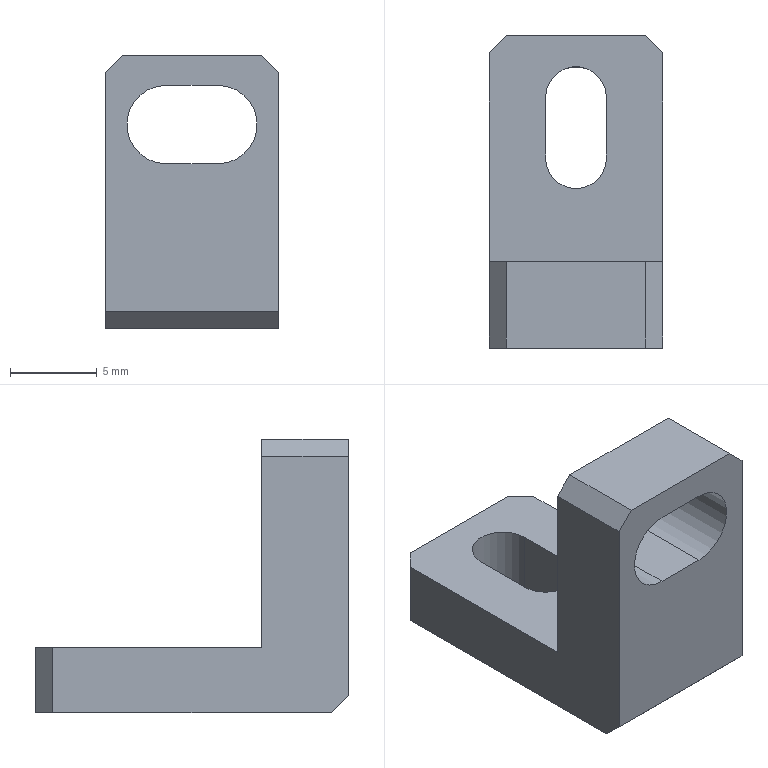Part | SolidWorks | features ICE 4, Chamfer 1, Extrusion 1 | 1 solid | 21 faces | box 10 x 18 x 15.75 mm | volume 1032 mm3 | plane 17 | cylinder 4 | commonest cylinder face diameters 3.5 x2 4.5 x2
STEP:
#1=CARTESIAN_POINT('',(0.,17.,-3.75));
#2=VERTEX_POINT('',#1);
#3=CARTESIAN_POINT('',(0.,1.,-3.75));
#4=VERTEX_POINT('',#3);
#5=CARTESIAN_POINT('',(0.,18.,-3.75));
#6=DIRECTION('',(0.,-1.,0.));
#7=VECTOR('',#6,1000.);
#8=LINE('',#5,#7);
#9=EDGE_CURVE('',#2,#4,#8,.T.);
#10=ORIENTED_EDGE('',*,*,#9,.T.);
#11=CARTESIAN_POINT('',(0.,0.,-2.75));
#12=VERTEX_POINT('',#11);
#13=CARTESIAN_POINT('',(0.,1.,-3.75));
#14=DIRECTION('',(0.,-0.7071,0.7071));
#15=VECTOR('',#14,1000.);
#16=LINE('',#13,#15);
#17=EDGE_CURVE('',#4,#12,#16,.T.);
#18=ORIENTED_EDGE('',*,*,#17,.T.);
#19=CARTESIAN_POINT('',(0.,0.,11.));
#20=VERTEX_POINT('',#19);
#21=CARTESIAN_POINT('',(0.,0.,0.));
#22=DIRECTION('',(0.,0.,1.));
#23=VECTOR('',#22,1000.);
#24=LINE('',#21,#23);
#25=EDGE_CURVE('',#12,#20,#24,.T.);
#26=ORIENTED_EDGE('',*,*,#25,.T.);
#27=CARTESIAN_POINT('',(0.,5.,11.));
#28=VERTEX_POINT('',#27);
#29=CARTESIAN_POINT('',(0.,5.,11.));
#30=DIRECTION('',(0.,1.,0.));
#31=VECTOR('',#30,1000.);
#32=LINE('',#29,#31);
#33=EDGE_CURVE('',#20,#28,#32,.T.);
#34=ORIENTED_EDGE('',*,*,#33,.T.);
#35=CARTESIAN_POINT('',(0.,5.,0.));
#36=VERTEX_POINT('',#35);
#37=CARTESIAN_POINT('',(0.,5.,0.));
#38=DIRECTION('',(0.,0.,-1.));
#39=VECTOR('',#38,1000.);
#40=LINE('',#37,#39);
#41=EDGE_CURVE('',#28,#36,#40,.T.);
#42=ORIENTED_EDGE('',*,*,#41,.T.);
#43=CARTESIAN_POINT('',(0.,17.,0.));
#44=VERTEX_POINT('',#43);
#45=CARTESIAN_POINT('',(0.,18.,0.));
#46=DIRECTION('',(0.,-1.,0.));
#47=VECTOR('',#46,1000.);
#48=LINE('',#45,#47);
#49=EDGE_CURVE('',#44,#36,#48,.T.);
#50=ORIENTED_EDGE('',*,*,#49,.F.);
#51=CARTESIAN_POINT('',(0.,17.,0.));
#52=DIRECTION('',(0.,0.,-1.));
#53=VECTOR('',#52,1000.);
#54=LINE('',#51,#53);
#55=EDGE_CURVE('',#44,#2,#54,.T.);
#56=ORIENTED_EDGE('',*,*,#55,.T.);
#57=EDGE_LOOP('',(#10,#18,#26,#34,#42,#50,#56));
#58=FACE_OUTER_BOUND('',#57,.T.);
#59=CARTESIAN_POINT('',(0.,18.,0.));
#60=DIRECTION('',(1.,0.,0.));
#61=DIRECTION('',(0.,0.,-1.));
#62=AXIS2_PLACEMENT_3D('',#59,#60,#61);
#63=PLANE('',#62);
#64=ADVANCED_FACE('',(#58),#63,.F.);
#65=CARTESIAN_POINT('',(3.25,14.45,0.));
#66=VERTEX_POINT('',#65);
#67=CARTESIAN_POINT('',(3.25,10.95,0.));
#68=VERTEX_POINT('',#67);
#69=CARTESIAN_POINT('',(3.25,14.45,0.));
#70=DIRECTION('',(0.,-1.,0.));
#71=VECTOR('',#70,1000.);
#72=LINE('',#69,#71);
#73=EDGE_CURVE('',#66,#68,#72,.T.);
#74=ORIENTED_EDGE('',*,*,#73,.F.);
#75=CARTESIAN_POINT('',(6.75,14.45,0.));
#76=VERTEX_POINT('',#75);
#77=CARTESIAN_POINT('',(5.,14.45,0.));
#78=DIRECTION('',(0.,0.,1.));
#79=DIRECTION('',(1.,0.,0.));
#80=AXIS2_PLACEMENT_3D('',#77,#78,#79);
#81=CIRCLE('',#80,1.75);
#82=EDGE_CURVE('',#76,#66,#81,.T.);
#83=ORIENTED_EDGE('',*,*,#82,.F.);
#84=CARTESIAN_POINT('',(6.75,10.95,0.));
#85=VERTEX_POINT('',#84);
#86=CARTESIAN_POINT('',(6.75,14.45,0.));
#87=DIRECTION('',(0.,1.,0.));
#88=VECTOR('',#87,1000.);
#89=LINE('',#86,#88);
#90=EDGE_CURVE('',#85,#76,#89,.T.);
#91=ORIENTED_EDGE('',*,*,#90,.F.);
#92=CARTESIAN_POINT('',(5.,10.95,0.));
#93=DIRECTION('',(0.,0.,1.));
#94=DIRECTION('',(1.,0.,0.));
#95=AXIS2_PLACEMENT_3D('',#92,#93,#94);
#96=CIRCLE('',#95,1.75);
#97=EDGE_CURVE('',#68,#85,#96,.T.);
#98=ORIENTED_EDGE('',*,*,#97,.F.);
#99=EDGE_LOOP('',(#74,#83,#91,#98));
#100=FACE_BOUND('',#99,.T.);
#101=CARTESIAN_POINT('',(10.,17.,0.));
#102=VERTEX_POINT('',#101);
#103=CARTESIAN_POINT('',(10.,5.,0.));
#104=VERTEX_POINT('',#103);
#105=CARTESIAN_POINT('',(10.,18.,0.));
#106=DIRECTION('',(0.,-1.,0.));
#107=VECTOR('',#106,1000.);
#108=LINE('',#105,#107);
#109=EDGE_CURVE('',#102,#104,#108,.T.);
#110=ORIENTED_EDGE('',*,*,#109,.F.);
#111=CARTESIAN_POINT('',(9.,18.,0.));
#112=VERTEX_POINT('',#111);
#113=CARTESIAN_POINT('',(9.,18.,0.));
#114=DIRECTION('',(-0.7071,0.7071,0.));
#115=VECTOR('',#114,1000.);
#116=LINE('',#113,#115);
#117=EDGE_CURVE('',#102,#112,#116,.T.);
#118=ORIENTED_EDGE('',*,*,#117,.T.);
#119=CARTESIAN_POINT('',(1.,18.,0.));
#120=VERTEX_POINT('',#119);
#121=CARTESIAN_POINT('',(0.,18.,0.));
#122=DIRECTION('',(1.,0.,0.));
#123=VECTOR('',#122,1000.);
#124=LINE('',#121,#123);
#125=EDGE_CURVE('',#120,#112,#124,.T.);
#126=ORIENTED_EDGE('',*,*,#125,.F.);
#127=CARTESIAN_POINT('',(1.,18.,0.));
#128=DIRECTION('',(-0.7071,-0.7071,0.));
#129=VECTOR('',#128,1000.);
#130=LINE('',#127,#129);
#131=EDGE_CURVE('',#120,#44,#130,.T.);
#132=ORIENTED_EDGE('',*,*,#131,.T.);
#133=ORIENTED_EDGE('',*,*,#49,.T.);
#134=CARTESIAN_POINT('',(0.,5.,0.));
#135=DIRECTION('',(1.,0.,0.));
#136=VECTOR('',#135,1000.);
#137=LINE('',#134,#136);
#138=EDGE_CURVE('',#36,#104,#137,.T.);
#139=ORIENTED_EDGE('',*,*,#138,.T.);
#140=EDGE_LOOP('',(#110,#118,#126,#132,#133,#139));
#141=FACE_OUTER_BOUND('',#140,.T.);
#142=CARTESIAN_POINT('',(0.,18.,0.));
#143=DIRECTION('',(0.,0.,-1.));
#144=DIRECTION('',(-1.,0.,0.));
#145=AXIS2_PLACEMENT_3D('',#142,#143,#144);
#146=PLANE('',#145);
#147=ADVANCED_FACE('',(#100,#141),#146,.F.);
#148=CARTESIAN_POINT('',(10.,0.,11.));
#149=VERTEX_POINT('',#148);
#150=CARTESIAN_POINT('',(10.,0.,-2.75));
#151=VERTEX_POINT('',#150);
#152=CARTESIAN_POINT('',(10.,0.,0.));
#153=DIRECTION('',(0.,0.,-1.));
#154=VECTOR('',#153,1000.);
#155=LINE('',#152,#154);
#156=EDGE_CURVE('',#149,#151,#155,.T.);
#157=ORIENTED_EDGE('',*,*,#156,.T.);
#158=CARTESIAN_POINT('',(10.,1.,-3.75));
#159=VERTEX_POINT('',#158);
#160=CARTESIAN_POINT('',(10.,1.,-3.75));
#161=DIRECTION('',(0.,0.7071,-0.7071));
#162=VECTOR('',#161,1000.);
#163=LINE('',#160,#162);
#164=EDGE_CURVE('',#151,#159,#163,.T.);
#165=ORIENTED_EDGE('',*,*,#164,.T.);
#166=CARTESIAN_POINT('',(10.,17.,-3.75));
#167=VERTEX_POINT('',#166);
#168=CARTESIAN_POINT('',(10.,18.,-3.75));
#169=DIRECTION('',(0.,-1.,0.));
#170=VECTOR('',#169,1000.);
#171=LINE('',#168,#170);
#172=EDGE_CURVE('',#167,#159,#171,.T.);
#173=ORIENTED_EDGE('',*,*,#172,.F.);
#174=CARTESIAN_POINT('',(10.,17.,0.));
#175=DIRECTION('',(0.,0.,1.));
#176=VECTOR('',#175,1000.);
#177=LINE('',#174,#176);
#178=EDGE_CURVE('',#167,#102,#177,.T.);
#179=ORIENTED_EDGE('',*,*,#178,.T.);
#180=ORIENTED_EDGE('',*,*,#109,.T.);
#181=CARTESIAN_POINT('',(10.,5.,11.));
#182=VERTEX_POINT('',#181);
#183=CARTESIAN_POINT('',(10.,5.,0.));
#184=DIRECTION('',(0.,0.,1.));
#185=VECTOR('',#184,1000.);
#186=LINE('',#183,#185);
#187=EDGE_CURVE('',#104,#182,#186,.T.);
#188=ORIENTED_EDGE('',*,*,#187,.T.);
#189=CARTESIAN_POINT('',(10.,0.,11.));
#190=DIRECTION('',(0.,-1.,0.));
#191=VECTOR('',#190,1000.);
#192=LINE('',#189,#191);
#193=EDGE_CURVE('',#182,#149,#192,.T.);
#194=ORIENTED_EDGE('',*,*,#193,.T.);
#195=EDGE_LOOP('',(#157,#165,#173,#179,#180,#188,#194));
#196=FACE_OUTER_BOUND('',#195,.T.);
#197=CARTESIAN_POINT('',(10.,18.,0.));
#198=DIRECTION('',(-1.,0.,0.));
#199=DIRECTION('',(0.,0.,1.));
#200=AXIS2_PLACEMENT_3D('',#197,#198,#199);
#201=PLANE('',#200);
#202=ADVANCED_FACE('',(#196),#201,.F.);
#203=CARTESIAN_POINT('',(6.75,10.95,-3.75));
#204=VERTEX_POINT('',#203);
#205=CARTESIAN_POINT('',(6.75,14.45,-3.75));
#206=VERTEX_POINT('',#205);
#207=CARTESIAN_POINT('',(6.75,18.,-3.75));
#208=DIRECTION('',(0.,1.,0.));
#209=VECTOR('',#208,1000.);
#210=LINE('',#207,#209);
#211=EDGE_CURVE('',#204,#206,#210,.T.);
#212=ORIENTED_EDGE('',*,*,#211,.T.);
#213=CARTESIAN_POINT('',(3.25,14.45,-3.75));
#214=VERTEX_POINT('',#213);
#215=CARTESIAN_POINT('',(5.,14.45,-3.75));
#216=DIRECTION('',(0.,0.,1.));
#217=DIRECTION('',(1.,0.,0.));
#218=AXIS2_PLACEMENT_3D('',#215,#216,#217);
#219=CIRCLE('',#218,1.75);
#220=EDGE_CURVE('',#206,#214,#219,.T.);
#221=ORIENTED_EDGE('',*,*,#220,.T.);
#222=CARTESIAN_POINT('',(3.25,10.95,-3.75));
#223=VERTEX_POINT('',#222);
#224=CARTESIAN_POINT('',(3.25,18.,-3.75));
#225=DIRECTION('',(0.,-1.,0.));
#226=VECTOR('',#225,1000.);
#227=LINE('',#224,#226);
#228=EDGE_CURVE('',#214,#223,#227,.T.);
#229=ORIENTED_EDGE('',*,*,#228,.T.);
#230=CARTESIAN_POINT('',(5.,10.95,-3.75));
#231=DIRECTION('',(0.,0.,1.));
#232=DIRECTION('',(1.,0.,0.));
#233=AXIS2_PLACEMENT_3D('',#230,#231,#232);
#234=CIRCLE('',#233,1.75);
#235=EDGE_CURVE('',#223,#204,#234,.T.);
#236=ORIENTED_EDGE('',*,*,#235,.T.);
#237=EDGE_LOOP('',(#212,#221,#229,#236));
#238=FACE_BOUND('',#237,.T.);
#239=ORIENTED_EDGE('',*,*,#172,.T.);
#240=CARTESIAN_POINT('',(0.,1.,-3.75));
#241=DIRECTION('',(-1.,0.,0.));
#242=VECTOR('',#241,1000.);
#243=LINE('',#240,#242);
#244=EDGE_CURVE('',#159,#4,#243,.T.);
#245=ORIENTED_EDGE('',*,*,#244,.T.);
#246=ORIENTED_EDGE('',*,*,#9,.F.);
#247=CARTESIAN_POINT('',(1.,18.,-3.75));
#248=VERTEX_POINT('',#247);
#249=CARTESIAN_POINT('',(1.,18.,-3.75));
#250=DIRECTION('',(0.7071,0.7071,0.));
#251=VECTOR('',#250,1000.);
#252=LINE('',#249,#251);
#253=EDGE_CURVE('',#2,#248,#252,.T.);
#254=ORIENTED_EDGE('',*,*,#253,.T.);
#255=CARTESIAN_POINT('',(9.,18.,-3.75));
#256=VERTEX_POINT('',#255);
#257=CARTESIAN_POINT('',(0.,18.,-3.75));
#258=DIRECTION('',(-1.,0.,0.));
#259=VECTOR('',#258,1000.);
#260=LINE('',#257,#259);
#261=EDGE_CURVE('',#256,#248,#260,.T.);
#262=ORIENTED_EDGE('',*,*,#261,.F.);
#263=CARTESIAN_POINT('',(9.,18.,-3.75));
#264=DIRECTION('',(0.7071,-0.7071,0.));
#265=VECTOR('',#264,1000.);
#266=LINE('',#263,#265);
#267=EDGE_CURVE('',#256,#167,#266,.T.);
#268=ORIENTED_EDGE('',*,*,#267,.T.);
#269=EDGE_LOOP('',(#239,#245,#246,#254,#262,#268));
#270=FACE_OUTER_BOUND('',#269,.T.);
#271=CARTESIAN_POINT('',(0.,18.,-3.75));
#272=DIRECTION('',(0.,0.,1.));
#273=DIRECTION('',(1.,0.,0.));
#274=AXIS2_PLACEMENT_3D('',#271,#272,#273);
#275=PLANE('',#274);
#276=ADVANCED_FACE('',(#238,#270),#275,.F.);
#277=ORIENTED_EDGE('',*,*,#125,.T.);
#278=CARTESIAN_POINT('',(9.,18.,0.));
#279=DIRECTION('',(0.,0.,-1.));
#280=VECTOR('',#279,1000.);
#281=LINE('',#278,#280);
#282=EDGE_CURVE('',#112,#256,#281,.T.);
#283=ORIENTED_EDGE('',*,*,#282,.T.);
#284=ORIENTED_EDGE('',*,*,#261,.T.);
#285=CARTESIAN_POINT('',(1.,18.,0.));
#286=DIRECTION('',(0.,0.,1.));
#287=VECTOR('',#286,1000.);
#288=LINE('',#285,#287);
#289=EDGE_CURVE('',#248,#120,#288,.T.);
#290=ORIENTED_EDGE('',*,*,#289,.T.);
#291=EDGE_LOOP('',(#277,#283,#284,#290));
#292=FACE_OUTER_BOUND('',#291,.T.);
#293=CARTESIAN_POINT('',(0.,18.,0.));
#294=DIRECTION('',(0.,-1.,0.));
#295=DIRECTION('',(0.,0.,-1.));
#296=AXIS2_PLACEMENT_3D('',#293,#294,#295);
#297=PLANE('',#296);
#298=ADVANCED_FACE('',(#292),#297,.F.);
#299=CARTESIAN_POINT('',(3.5,0.,10.25));
#300=VERTEX_POINT('',#299);
#301=CARTESIAN_POINT('',(3.5,0.,5.75));
#302=VERTEX_POINT('',#301);
#303=CARTESIAN_POINT('',(3.5,0.,8.));
#304=DIRECTION('',(0.,-1.,0.));
#305=DIRECTION('',(0.,0.,-1.));
#306=AXIS2_PLACEMENT_3D('',#303,#304,#305);
#307=CIRCLE('',#306,2.25);
#308=EDGE_CURVE('',#300,#302,#307,.T.);
#309=ORIENTED_EDGE('',*,*,#308,.F.);
#310=CARTESIAN_POINT('',(6.5,0.,10.25));
#311=VERTEX_POINT('',#310);
#312=CARTESIAN_POINT('',(0.,0.,10.25));
#313=DIRECTION('',(-1.,0.,0.));
#314=VECTOR('',#313,1000.);
#315=LINE('',#312,#314);
#316=EDGE_CURVE('',#311,#300,#315,.T.);
#317=ORIENTED_EDGE('',*,*,#316,.F.);
#318=CARTESIAN_POINT('',(6.5,0.,5.75));
#319=VERTEX_POINT('',#318);
#320=CARTESIAN_POINT('',(6.5,0.,8.));
#321=DIRECTION('',(0.,-1.,0.));
#322=DIRECTION('',(0.,0.,-1.));
#323=AXIS2_PLACEMENT_3D('',#320,#321,#322);
#324=CIRCLE('',#323,2.25);
#325=EDGE_CURVE('',#319,#311,#324,.T.);
#326=ORIENTED_EDGE('',*,*,#325,.F.);
#327=CARTESIAN_POINT('',(0.,0.,5.75));
#328=DIRECTION('',(1.,0.,0.));
#329=VECTOR('',#328,1000.);
#330=LINE('',#327,#329);
#331=EDGE_CURVE('',#302,#319,#330,.T.);
#332=ORIENTED_EDGE('',*,*,#331,.F.);
#333=EDGE_LOOP('',(#309,#317,#326,#332));
#334=FACE_BOUND('',#333,.T.);
#335=ORIENTED_EDGE('',*,*,#25,.F.);
#336=CARTESIAN_POINT('',(10.,0.,-2.75));
#337=DIRECTION('',(1.,0.,0.));
#338=VECTOR('',#337,1000.);
#339=LINE('',#336,#338);
#340=EDGE_CURVE('',#12,#151,#339,.T.);
#341=ORIENTED_EDGE('',*,*,#340,.T.);
#342=ORIENTED_EDGE('',*,*,#156,.F.);
#343=CARTESIAN_POINT('',(9.,0.,12.));
#344=VERTEX_POINT('',#343);
#345=CARTESIAN_POINT('',(10.5,0.,10.5));
#346=DIRECTION('',(-0.7071,0.,0.7071));
#347=VECTOR('',#346,1000.);
#348=LINE('',#345,#347);
#349=EDGE_CURVE('',#149,#344,#348,.T.);
#350=ORIENTED_EDGE('',*,*,#349,.T.);
#351=CARTESIAN_POINT('',(1.,0.,12.));
#352=VERTEX_POINT('',#351);
#353=CARTESIAN_POINT('',(0.,0.,12.));
#354=DIRECTION('',(-1.,0.,0.));
#355=VECTOR('',#354,1000.);
#356=LINE('',#353,#355);
#357=EDGE_CURVE('',#344,#352,#356,.T.);
#358=ORIENTED_EDGE('',*,*,#357,.T.);
#359=CARTESIAN_POINT('',(-5.5,0.,5.5));
#360=DIRECTION('',(-0.7071,0.,-0.7071));
#361=VECTOR('',#360,1000.);
#362=LINE('',#359,#361);
#363=EDGE_CURVE('',#352,#20,#362,.T.);
#364=ORIENTED_EDGE('',*,*,#363,.T.);
#365=EDGE_LOOP('',(#335,#341,#342,#350,#358,#364));
#366=FACE_OUTER_BOUND('',#365,.T.);
#367=CARTESIAN_POINT('',(0.,0.,0.));
#368=DIRECTION('',(0.,-1.,0.));
#369=DIRECTION('',(0.,0.,-1.));
#370=AXIS2_PLACEMENT_3D('',#367,#368,#369);
#371=PLANE('',#370);
#372=ADVANCED_FACE('',(#334,#366),#371,.T.);
#373=CARTESIAN_POINT('',(9.,5.,12.));
#374=VERTEX_POINT('',#373);
#375=CARTESIAN_POINT('',(1.,5.,12.));
#376=VERTEX_POINT('',#375);
#377=CARTESIAN_POINT('',(0.,5.,12.));
#378=DIRECTION('',(-1.,0.,0.));
#379=VECTOR('',#378,1000.);
#380=LINE('',#377,#379);
#381=EDGE_CURVE('',#374,#376,#380,.T.);
#382=ORIENTED_EDGE('',*,*,#381,.T.);
#383=CARTESIAN_POINT('',(1.,0.,12.));
#384=DIRECTION('',(0.,-1.,0.));
#385=VECTOR('',#384,1000.);
#386=LINE('',#383,#385);
#387=EDGE_CURVE('',#376,#352,#386,.T.);
#388=ORIENTED_EDGE('',*,*,#387,.T.);
#389=ORIENTED_EDGE('',*,*,#357,.F.);
#390=CARTESIAN_POINT('',(9.,5.,12.));
#391=DIRECTION('',(0.,1.,0.));
#392=VECTOR('',#391,1000.);
#393=LINE('',#390,#392);
#394=EDGE_CURVE('',#344,#374,#393,.T.);
#395=ORIENTED_EDGE('',*,*,#394,.T.);
#396=EDGE_LOOP('',(#382,#388,#389,#395));
#397=FACE_OUTER_BOUND('',#396,.T.);
#398=CARTESIAN_POINT('',(0.,5.,12.));
#399=DIRECTION('',(0.,0.,1.));
#400=DIRECTION('',(1.,0.,0.));
#401=AXIS2_PLACEMENT_3D('',#398,#399,#400);
#402=PLANE('',#401);
#403=ADVANCED_FACE('',(#397),#402,.T.);
#404=CARTESIAN_POINT('',(3.5,5.,5.75));
#405=VERTEX_POINT('',#404);
#406=CARTESIAN_POINT('',(3.5,5.,10.25));
#407=VERTEX_POINT('',#406);
#408=CARTESIAN_POINT('',(3.5,5.,8.));
#409=DIRECTION('',(0.,1.,0.));
#410=DIRECTION('',(0.,0.,1.));
#411=AXIS2_PLACEMENT_3D('',#408,#409,#410);
#412=CIRCLE('',#411,2.25);
#413=EDGE_CURVE('',#405,#407,#412,.T.);
#414=ORIENTED_EDGE('',*,*,#413,.F.);
#415=CARTESIAN_POINT('',(6.5,5.,5.75));
#416=VERTEX_POINT('',#415);
#417=CARTESIAN_POINT('',(3.5,5.,5.75));
#418=DIRECTION('',(-1.,0.,0.));
#419=VECTOR('',#418,1000.);
#420=LINE('',#417,#419);
#421=EDGE_CURVE('',#416,#405,#420,.T.);
#422=ORIENTED_EDGE('',*,*,#421,.F.);
#423=CARTESIAN_POINT('',(6.5,5.,10.25));
#424=VERTEX_POINT('',#423);
#425=CARTESIAN_POINT('',(6.5,5.,8.));
#426=DIRECTION('',(0.,1.,0.));
#427=DIRECTION('',(0.,0.,1.));
#428=AXIS2_PLACEMENT_3D('',#425,#426,#427);
#429=CIRCLE('',#428,2.25);
#430=EDGE_CURVE('',#424,#416,#429,.T.);
#431=ORIENTED_EDGE('',*,*,#430,.F.);
#432=CARTESIAN_POINT('',(3.5,5.,10.25));
#433=DIRECTION('',(1.,0.,0.));
#434=VECTOR('',#433,1000.);
#435=LINE('',#432,#434);
#436=EDGE_CURVE('',#407,#424,#435,.T.);
#437=ORIENTED_EDGE('',*,*,#436,.F.);
#438=EDGE_LOOP('',(#414,#422,#431,#437));
#439=FACE_BOUND('',#438,.T.);
#440=ORIENTED_EDGE('',*,*,#41,.F.);
#441=CARTESIAN_POINT('',(-5.5,5.,5.5));
#442=DIRECTION('',(0.7071,0.,0.7071));
#443=VECTOR('',#442,1000.);
#444=LINE('',#441,#443);
#445=EDGE_CURVE('',#28,#376,#444,.T.);
#446=ORIENTED_EDGE('',*,*,#445,.T.);
#447=ORIENTED_EDGE('',*,*,#381,.F.);
#448=CARTESIAN_POINT('',(10.5,5.,10.5));
#449=DIRECTION('',(0.7071,0.,-0.7071));
#450=VECTOR('',#449,1000.);
#451=LINE('',#448,#450);
#452=EDGE_CURVE('',#374,#182,#451,.T.);
#453=ORIENTED_EDGE('',*,*,#452,.T.);
#454=ORIENTED_EDGE('',*,*,#187,.F.);
#455=ORIENTED_EDGE('',*,*,#138,.F.);
#456=EDGE_LOOP('',(#440,#446,#447,#453,#454,#455));
#457=FACE_OUTER_BOUND('',#456,.T.);
#458=CARTESIAN_POINT('',(0.,5.,0.));
#459=DIRECTION('',(0.,1.,0.));
#460=DIRECTION('',(0.,0.,1.));
#461=AXIS2_PLACEMENT_3D('',#458,#459,#460);
#462=PLANE('',#461);
#463=ADVANCED_FACE('',(#439,#457),#462,.T.);
#464=ORIENTED_EDGE('',*,*,#308,.T.);
#465=CARTESIAN_POINT('',(3.5,-5.,5.75));
#466=DIRECTION('',(0.,1.,0.));
#467=VECTOR('',#466,1000.);
#468=LINE('',#465,#467);
#469=EDGE_CURVE('',#302,#405,#468,.T.);
#470=ORIENTED_EDGE('',*,*,#469,.T.);
#471=ORIENTED_EDGE('',*,*,#413,.T.);
#472=CARTESIAN_POINT('',(3.5,-5.,10.25));
#473=DIRECTION('',(0.,1.,0.));
#474=VECTOR('',#473,1000.);
#475=LINE('',#472,#474);
#476=EDGE_CURVE('',#300,#407,#475,.T.);
#477=ORIENTED_EDGE('',*,*,#476,.F.);
#478=EDGE_LOOP('',(#464,#470,#471,#477));
#479=FACE_OUTER_BOUND('',#478,.T.);
#480=CARTESIAN_POINT('',(3.5,-5.,8.));
#481=DIRECTION('',(0.,1.,0.));
#482=DIRECTION('',(0.,0.,1.));
#483=AXIS2_PLACEMENT_3D('',#480,#481,#482);
#484=CYLINDRICAL_SURFACE('',#483,2.25);
#485=ADVANCED_FACE('',(#479),#484,.F.);
#486=ORIENTED_EDGE('',*,*,#331,.T.);
#487=CARTESIAN_POINT('',(6.5,-5.,5.75));
#488=DIRECTION('',(0.,1.,0.));
#489=VECTOR('',#488,1000.);
#490=LINE('',#487,#489);
#491=EDGE_CURVE('',#319,#416,#490,.T.);
#492=ORIENTED_EDGE('',*,*,#491,.T.);
#493=ORIENTED_EDGE('',*,*,#421,.T.);
#494=ORIENTED_EDGE('',*,*,#469,.F.);
#495=EDGE_LOOP('',(#486,#492,#493,#494));
#496=FACE_OUTER_BOUND('',#495,.T.);
#497=CARTESIAN_POINT('',(3.5,-5.,5.75));
#498=DIRECTION('',(0.,0.,-1.));
#499=DIRECTION('',(-1.,0.,0.));
#500=AXIS2_PLACEMENT_3D('',#497,#498,#499);
#501=PLANE('',#500);
#502=ADVANCED_FACE('',(#496),#501,.F.);
#503=ORIENTED_EDGE('',*,*,#325,.T.);
#504=CARTESIAN_POINT('',(6.5,-5.,10.25));
#505=DIRECTION('',(0.,1.,0.));
#506=VECTOR('',#505,1000.);
#507=LINE('',#504,#506);
#508=EDGE_CURVE('',#311,#424,#507,.T.);
#509=ORIENTED_EDGE('',*,*,#508,.T.);
#510=ORIENTED_EDGE('',*,*,#430,.T.);
#511=ORIENTED_EDGE('',*,*,#491,.F.);
#512=EDGE_LOOP('',(#503,#509,#510,#511));
#513=FACE_OUTER_BOUND('',#512,.T.);
#514=CARTESIAN_POINT('',(6.5,-5.,8.));
#515=DIRECTION('',(0.,1.,0.));
#516=DIRECTION('',(0.,0.,1.));
#517=AXIS2_PLACEMENT_3D('',#514,#515,#516);
#518=CYLINDRICAL_SURFACE('',#517,2.25);
#519=ADVANCED_FACE('',(#513),#518,.F.);
#520=ORIENTED_EDGE('',*,*,#316,.T.);
#521=ORIENTED_EDGE('',*,*,#476,.T.);
#522=ORIENTED_EDGE('',*,*,#436,.T.);
#523=ORIENTED_EDGE('',*,*,#508,.F.);
#524=EDGE_LOOP('',(#520,#521,#522,#523));
#525=FACE_OUTER_BOUND('',#524,.T.);
#526=CARTESIAN_POINT('',(3.5,-5.,10.25));
#527=DIRECTION('',(0.,0.,1.));
#528=DIRECTION('',(1.,0.,0.));
#529=AXIS2_PLACEMENT_3D('',#526,#527,#528);
#530=PLANE('',#529);
#531=ADVANCED_FACE('',(#525),#530,.F.);
#532=ORIENTED_EDGE('',*,*,#164,.F.);
#533=ORIENTED_EDGE('',*,*,#340,.F.);
#534=ORIENTED_EDGE('',*,*,#17,.F.);
#535=ORIENTED_EDGE('',*,*,#244,.F.);
#536=EDGE_LOOP('',(#532,#533,#534,#535));
#537=FACE_OUTER_BOUND('',#536,.T.);
#538=CARTESIAN_POINT('',(0.,1.,-3.75));
#539=DIRECTION('',(0.,-0.7071,-0.7071));
#540=DIRECTION('',(1.,0.,0.));
#541=AXIS2_PLACEMENT_3D('',#538,#539,#540);
#542=PLANE('',#541);
#543=ADVANCED_FACE('',(#537),#542,.T.);
#544=ORIENTED_EDGE('',*,*,#117,.F.);
#545=ORIENTED_EDGE('',*,*,#178,.F.);
#546=ORIENTED_EDGE('',*,*,#267,.F.);
#547=ORIENTED_EDGE('',*,*,#282,.F.);
#548=EDGE_LOOP('',(#544,#545,#546,#547));
#549=FACE_OUTER_BOUND('',#548,.T.);
#550=CARTESIAN_POINT('',(9.,18.,0.));
#551=DIRECTION('',(-0.7071,-0.7071,0.));
#552=DIRECTION('',(0.,0.,-1.));
#553=AXIS2_PLACEMENT_3D('',#550,#551,#552);
#554=PLANE('',#553);
#555=ADVANCED_FACE('',(#549),#554,.F.);
#556=ORIENTED_EDGE('',*,*,#253,.F.);
#557=ORIENTED_EDGE('',*,*,#55,.F.);
#558=ORIENTED_EDGE('',*,*,#131,.F.);
#559=ORIENTED_EDGE('',*,*,#289,.F.);
#560=EDGE_LOOP('',(#556,#557,#558,#559));
#561=FACE_OUTER_BOUND('',#560,.T.);
#562=CARTESIAN_POINT('',(1.,18.,0.));
#563=DIRECTION('',(0.7071,-0.7071,0.));
#564=DIRECTION('',(0.,0.,1.));
#565=AXIS2_PLACEMENT_3D('',#562,#563,#564);
#566=PLANE('',#565);
#567=ADVANCED_FACE('',(#561),#566,.F.);
#568=ORIENTED_EDGE('',*,*,#445,.F.);
#569=ORIENTED_EDGE('',*,*,#33,.F.);
#570=ORIENTED_EDGE('',*,*,#363,.F.);
#571=ORIENTED_EDGE('',*,*,#387,.F.);
#572=EDGE_LOOP('',(#568,#569,#570,#571));
#573=FACE_OUTER_BOUND('',#572,.T.);
#574=CARTESIAN_POINT('',(1.,5.,12.));
#575=DIRECTION('',(-0.7071,0.,0.7071));
#576=DIRECTION('',(0.,1.,0.));
#577=AXIS2_PLACEMENT_3D('',#574,#575,#576);
#578=PLANE('',#577);
#579=ADVANCED_FACE('',(#573),#578,.T.);
#580=ORIENTED_EDGE('',*,*,#452,.F.);
#581=ORIENTED_EDGE('',*,*,#394,.F.);
#582=ORIENTED_EDGE('',*,*,#349,.F.);
#583=ORIENTED_EDGE('',*,*,#193,.F.);
#584=EDGE_LOOP('',(#580,#581,#582,#583));
#585=FACE_OUTER_BOUND('',#584,.T.);
#586=CARTESIAN_POINT('',(10.,18.,11.));
#587=DIRECTION('',(0.7071,0.,0.7071));
#588=DIRECTION('',(0.,1.,0.));
#589=AXIS2_PLACEMENT_3D('',#586,#587,#588);
#590=PLANE('',#589);
#591=ADVANCED_FACE('',(#585),#590,.T.);
#592=CARTESIAN_POINT('',(6.75,14.45,-10.));
#593=DIRECTION('',(0.,0.,1.));
#594=VECTOR('',#593,1000.);
#595=LINE('',#592,#594);
#596=EDGE_CURVE('',#206,#76,#595,.T.);
#597=ORIENTED_EDGE('',*,*,#596,.T.);
#598=ORIENTED_EDGE('',*,*,#82,.T.);
#599=CARTESIAN_POINT('',(3.25,14.45,-10.));
#600=DIRECTION('',(0.,0.,1.));
#601=VECTOR('',#600,1000.);
#602=LINE('',#599,#601);
#603=EDGE_CURVE('',#214,#66,#602,.T.);
#604=ORIENTED_EDGE('',*,*,#603,.F.);
#605=ORIENTED_EDGE('',*,*,#220,.F.);
#606=EDGE_LOOP('',(#597,#598,#604,#605));
#607=FACE_OUTER_BOUND('',#606,.T.);
#608=CARTESIAN_POINT('',(5.,14.45,-10.));
#609=DIRECTION('',(0.,0.,1.));
#610=DIRECTION('',(1.,0.,0.));
#611=AXIS2_PLACEMENT_3D('',#608,#609,#610);
#612=CYLINDRICAL_SURFACE('',#611,1.75);
#613=ADVANCED_FACE('',(#607),#612,.F.);
#614=CARTESIAN_POINT('',(3.25,10.95,-10.));
#615=DIRECTION('',(0.,0.,1.));
#616=VECTOR('',#615,1000.);
#617=LINE('',#614,#616);
#618=EDGE_CURVE('',#223,#68,#617,.T.);
#619=ORIENTED_EDGE('',*,*,#618,.T.);
#620=ORIENTED_EDGE('',*,*,#97,.T.);
#621=CARTESIAN_POINT('',(6.75,10.95,-10.));
#622=DIRECTION('',(0.,0.,1.));
#623=VECTOR('',#622,1000.);
#624=LINE('',#621,#623);
#625=EDGE_CURVE('',#204,#85,#624,.T.);
#626=ORIENTED_EDGE('',*,*,#625,.F.);
#627=ORIENTED_EDGE('',*,*,#235,.F.);
#628=EDGE_LOOP('',(#619,#620,#626,#627));
#629=FACE_OUTER_BOUND('',#628,.T.);
#630=CARTESIAN_POINT('',(5.,10.95,-10.));
#631=DIRECTION('',(0.,0.,1.));
#632=DIRECTION('',(1.,0.,0.));
#633=AXIS2_PLACEMENT_3D('',#630,#631,#632);
#634=CYLINDRICAL_SURFACE('',#633,1.75);
#635=ADVANCED_FACE('',(#629),#634,.F.);
#636=ORIENTED_EDGE('',*,*,#625,.T.);
#637=ORIENTED_EDGE('',*,*,#90,.T.);
#638=ORIENTED_EDGE('',*,*,#596,.F.);
#639=ORIENTED_EDGE('',*,*,#211,.F.);
#640=EDGE_LOOP('',(#636,#637,#638,#639));
#641=FACE_OUTER_BOUND('',#640,.T.);
#642=CARTESIAN_POINT('',(6.75,14.45,-10.));
#643=DIRECTION('',(1.,0.,0.));
#644=DIRECTION('',(0.,1.,0.));
#645=AXIS2_PLACEMENT_3D('',#642,#643,#644);
#646=PLANE('',#645);
#647=ADVANCED_FACE('',(#641),#646,.F.);
#648=ORIENTED_EDGE('',*,*,#603,.T.);
#649=ORIENTED_EDGE('',*,*,#73,.T.);
#650=ORIENTED_EDGE('',*,*,#618,.F.);
#651=ORIENTED_EDGE('',*,*,#228,.F.);
#652=EDGE_LOOP('',(#648,#649,#650,#651));
#653=FACE_OUTER_BOUND('',#652,.T.);
#654=CARTESIAN_POINT('',(3.25,14.45,-10.));
#655=DIRECTION('',(-1.,0.,0.));
#656=DIRECTION('',(0.,-1.,0.));
#657=AXIS2_PLACEMENT_3D('',#654,#655,#656);
#658=PLANE('',#657);
#659=ADVANCED_FACE('',(#653),#658,.F.);
#660=CLOSED_SHELL('',(#64,#147,#202,#276,#298,#372,#403,#463,#485,#502,#519,#531,#543,#555,#567,#579,#591,#613,#635,#647,#659));
#661=MANIFOLD_SOLID_BREP('',#660);
#662=CARTESIAN_POINT('',(0.,0.,0.));
#663=DIRECTION('',(0.,0.,1.));
#664=DIRECTION('',(1.,0.,0.));
#665=AXIS2_PLACEMENT_3D('',#662,#663,#664);
#666=(LENGTH_UNIT()NAMED_UNIT(*)SI_UNIT(.MILLI.,.METRE.));
#667=UNCERTAINTY_MEASURE_WITH_UNIT(LENGTH_MEASURE(0.00001),#666,'','');
#668=(NAMED_UNIT(*)PLANE_ANGLE_UNIT()SI_UNIT($,.RADIAN.));
#669=(NAMED_UNIT(*)SI_UNIT($,.STERADIAN.)SOLID_ANGLE_UNIT());
#670=(GEOMETRIC_REPRESENTATION_CONTEXT(3)GLOBAL_UNCERTAINTY_ASSIGNED_CONTEXT((#667))GLOBAL_UNIT_ASSIGNED_CONTEXT((#666,#668,#669))REPRESENTATION_CONTEXT('',''));
#671=ADVANCED_BREP_SHAPE_REPRESENTATION('',(#661,#665),#670);